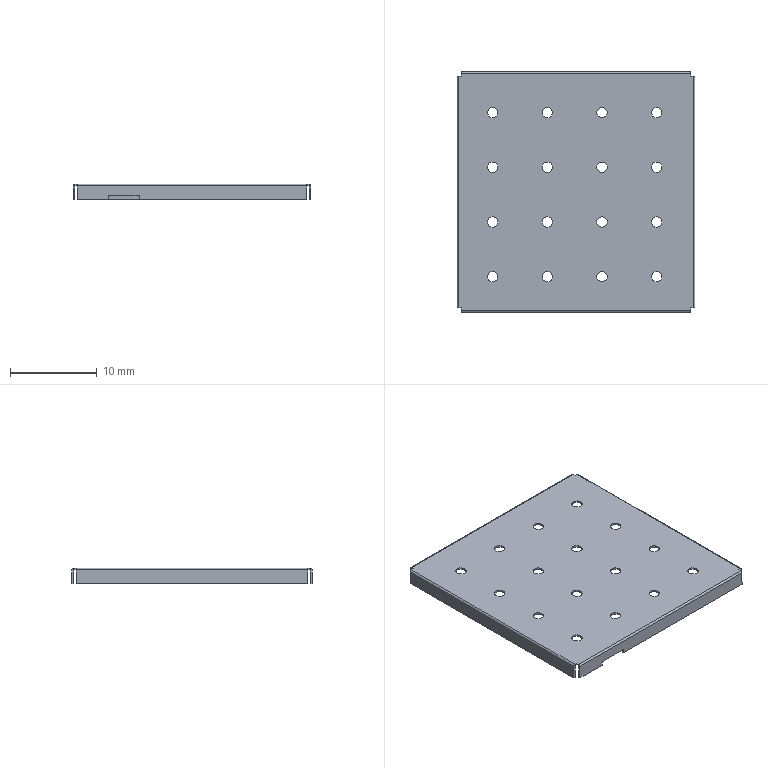Part | Creo | 1 solid | 62 faces | box 27.4 x 27.7 x 1.8 mm | volume 180.699 mm3 | cylinder 36 | plane 26 | commonest cylinder face diameters 1.2 x32 0.4 x4